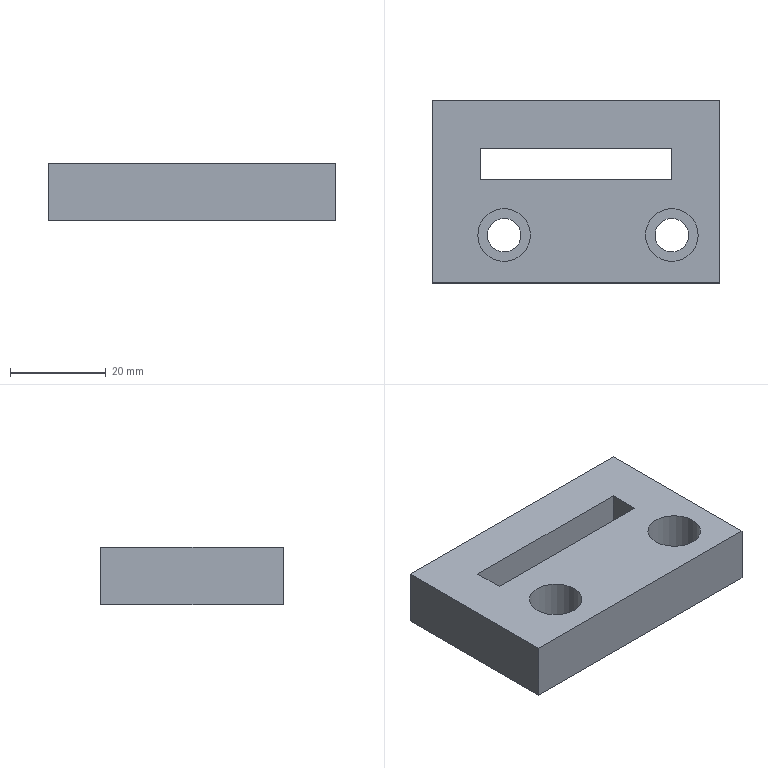Part | STEP file | lll_id682_x_t | 1 solid | 16 faces | box 60 x 38 x 12 mm | volume 22481 mm3 | plane 12 | cylinder 4 | commonest cylinder face diameters 7.009 x2 11.008 x2
STEP:
#1=CARTESIAN_POINT('',(359.5,-168.675,-12.));
#2=VERTEX_POINT('',#1);
#3=CARTESIAN_POINT('',(359.5,-162.325,-12.));
#4=VERTEX_POINT('',#3);
#5=CARTESIAN_POINT('',(359.5,-168.675,-12.));
#6=DIRECTION('',(0.,1.,0.));
#7=VECTOR('',#6,1.);
#8=LINE('',#5,#7);
#9=EDGE_CURVE('',#2,#4,#8,.T.);
#10=ORIENTED_EDGE('',*,*,#9,.T.);
#11=CARTESIAN_POINT('',(319.5,-162.325,-12.));
#12=VERTEX_POINT('',#11);
#13=CARTESIAN_POINT('',(339.5,-162.325,-12.));
#14=DIRECTION('',(-1.,0.,0.));
#15=VECTOR('',#14,1.);
#16=LINE('',#13,#15);
#17=EDGE_CURVE('',#4,#12,#16,.T.);
#18=ORIENTED_EDGE('',*,*,#17,.T.);
#19=CARTESIAN_POINT('',(319.5,-168.675,-12.));
#20=VERTEX_POINT('',#19);
#21=CARTESIAN_POINT('',(319.5,-168.675,-12.));
#22=DIRECTION('',(0.,1.,0.));
#23=VECTOR('',#22,1.);
#24=LINE('',#21,#23);
#25=EDGE_CURVE('',#20,#12,#24,.T.);
#26=ORIENTED_EDGE('',*,*,#25,.F.);
#27=CARTESIAN_POINT('',(339.5,-168.675,-12.));
#28=DIRECTION('',(-1.,0.,0.));
#29=VECTOR('',#28,1.);
#30=LINE('',#27,#29);
#31=EDGE_CURVE('',#2,#20,#30,.T.);
#32=ORIENTED_EDGE('',*,*,#31,.F.);
#33=EDGE_LOOP('',(#10,#18,#26,#32));
#34=FACE_BOUND('',#33,.T.);
#35=CARTESIAN_POINT('',(369.505,-190.325,-12.));
#36=VERTEX_POINT('',#35);
#37=CARTESIAN_POINT('',(369.505,-152.325,-12.));
#38=VERTEX_POINT('',#37);
#39=CARTESIAN_POINT('',(369.505,-165.5,-12.));
#40=DIRECTION('',(0.,1.,0.));
#41=VECTOR('',#40,1.);
#42=LINE('',#39,#41);
#43=EDGE_CURVE('',#36,#38,#42,.T.);
#44=ORIENTED_EDGE('',*,*,#43,.F.);
#45=CARTESIAN_POINT('',(309.505,-190.325,-12.));
#46=VERTEX_POINT('',#45);
#47=CARTESIAN_POINT('',(44.,-190.325,-12.));
#48=DIRECTION('',(1.,0.,0.));
#49=VECTOR('',#48,1.);
#50=LINE('',#47,#49);
#51=EDGE_CURVE('',#46,#36,#50,.T.);
#52=ORIENTED_EDGE('',*,*,#51,.F.);
#53=CARTESIAN_POINT('',(309.505,-152.325,-12.));
#54=VERTEX_POINT('',#53);
#55=CARTESIAN_POINT('',(309.505,-165.5,-12.));
#56=DIRECTION('',(0.,-1.,0.));
#57=VECTOR('',#56,1.);
#58=LINE('',#55,#57);
#59=EDGE_CURVE('',#54,#46,#58,.T.);
#60=ORIENTED_EDGE('',*,*,#59,.F.);
#61=CARTESIAN_POINT('',(44.,-152.325,-12.));
#62=DIRECTION('',(-1.,0.,0.));
#63=VECTOR('',#62,1.);
#64=LINE('',#61,#63);
#65=EDGE_CURVE('',#38,#54,#64,.T.);
#66=ORIENTED_EDGE('',*,*,#65,.F.);
#67=EDGE_LOOP('',(#44,#52,#60,#66));
#68=FACE_BOUND('',#67,.T.);
#69=CARTESIAN_POINT('',(328.009,-180.325,-12.));
#70=VERTEX_POINT('',#69);
#71=CARTESIAN_POINT('',(324.505,-180.325,-12.));
#72=DIRECTION('',(0.,0.,-1.));
#73=DIRECTION('',(1.,0.,0.));
#74=AXIS2_PLACEMENT_3D('',#71,#72,#73);
#75=CIRCLE('',#74,3.505);
#76=EDGE_CURVE('',#70,#70,#75,.T.);
#77=ORIENTED_EDGE('',*,*,#76,.F.);
#78=EDGE_LOOP('',(#77));
#79=FACE_BOUND('',#78,.T.);
#80=CARTESIAN_POINT('',(356.,-180.325,-12.));
#81=VERTEX_POINT('',#80);
#82=CARTESIAN_POINT('',(359.505,-180.325,-12.));
#83=DIRECTION('',(0.,0.,1.));
#84=DIRECTION('',(-1.,0.,0.));
#85=AXIS2_PLACEMENT_3D('',#82,#83,#84);
#86=CIRCLE('',#85,3.505);
#87=EDGE_CURVE('',#81,#81,#86,.T.);
#88=ORIENTED_EDGE('',*,*,#87,.T.);
#89=EDGE_LOOP('',(#88));
#90=FACE_BOUND('',#89,.T.);
#91=CARTESIAN_POINT('',(329.505,-165.5,-12.));
#92=DIRECTION('',(0.,0.,-1.));
#93=DIRECTION('',(1.,0.,0.));
#94=AXIS2_PLACEMENT_3D('',#91,#92,#93);
#95=PLANE('',#94);
#96=ADVANCED_FACE('',(#34,#68,#79,#90),#95,.T.);
#97=CARTESIAN_POINT('',(369.505,-190.325,0.));
#98=VERTEX_POINT('',#97);
#99=CARTESIAN_POINT('',(309.505,-190.325,0.));
#100=VERTEX_POINT('',#99);
#101=CARTESIAN_POINT('',(44.,-190.325,0.));
#102=DIRECTION('',(-1.,0.,0.));
#103=VECTOR('',#102,1.);
#104=LINE('',#101,#103);
#105=EDGE_CURVE('',#98,#100,#104,.T.);
#106=ORIENTED_EDGE('',*,*,#105,.F.);
#107=CARTESIAN_POINT('',(369.505,-152.325,0.));
#108=VERTEX_POINT('',#107);
#109=CARTESIAN_POINT('',(369.505,-165.5,0.));
#110=DIRECTION('',(0.,-1.,0.));
#111=VECTOR('',#110,1.);
#112=LINE('',#109,#111);
#113=EDGE_CURVE('',#108,#98,#112,.T.);
#114=ORIENTED_EDGE('',*,*,#113,.F.);
#115=CARTESIAN_POINT('',(309.505,-152.325,0.));
#116=VERTEX_POINT('',#115);
#117=CARTESIAN_POINT('',(44.,-152.325,0.));
#118=DIRECTION('',(1.,0.,0.));
#119=VECTOR('',#118,1.);
#120=LINE('',#117,#119);
#121=EDGE_CURVE('',#116,#108,#120,.T.);
#122=ORIENTED_EDGE('',*,*,#121,.F.);
#123=CARTESIAN_POINT('',(309.505,-165.5,0.));
#124=DIRECTION('',(0.,1.,0.));
#125=VECTOR('',#124,1.);
#126=LINE('',#123,#125);
#127=EDGE_CURVE('',#100,#116,#126,.T.);
#128=ORIENTED_EDGE('',*,*,#127,.F.);
#129=EDGE_LOOP('',(#106,#114,#122,#128));
#130=FACE_BOUND('',#129,.T.);
#131=CARTESIAN_POINT('',(359.5,-162.325,0.));
#132=VERTEX_POINT('',#131);
#133=CARTESIAN_POINT('',(319.5,-162.325,0.));
#134=VERTEX_POINT('',#133);
#135=CARTESIAN_POINT('',(339.5,-162.325,0.));
#136=DIRECTION('',(-1.,0.,0.));
#137=VECTOR('',#136,1.);
#138=LINE('',#135,#137);
#139=EDGE_CURVE('',#132,#134,#138,.T.);
#140=ORIENTED_EDGE('',*,*,#139,.F.);
#141=CARTESIAN_POINT('',(359.5,-168.675,0.));
#142=VERTEX_POINT('',#141);
#143=CARTESIAN_POINT('',(359.5,-168.675,0.));
#144=DIRECTION('',(0.,1.,0.));
#145=VECTOR('',#144,1.);
#146=LINE('',#143,#145);
#147=EDGE_CURVE('',#142,#132,#146,.T.);
#148=ORIENTED_EDGE('',*,*,#147,.F.);
#149=CARTESIAN_POINT('',(319.5,-168.675,0.));
#150=VERTEX_POINT('',#149);
#151=CARTESIAN_POINT('',(339.5,-168.675,0.));
#152=DIRECTION('',(-1.,0.,0.));
#153=VECTOR('',#152,1.);
#154=LINE('',#151,#153);
#155=EDGE_CURVE('',#142,#150,#154,.T.);
#156=ORIENTED_EDGE('',*,*,#155,.T.);
#157=CARTESIAN_POINT('',(319.5,-168.675,0.));
#158=DIRECTION('',(0.,1.,0.));
#159=VECTOR('',#158,1.);
#160=LINE('',#157,#159);
#161=EDGE_CURVE('',#150,#134,#160,.T.);
#162=ORIENTED_EDGE('',*,*,#161,.T.);
#163=EDGE_LOOP('',(#140,#148,#156,#162));
#164=FACE_BOUND('',#163,.T.);
#165=CARTESIAN_POINT('',(330.009,-180.325,0.));
#166=VERTEX_POINT('',#165);
#167=CARTESIAN_POINT('',(324.505,-180.325,0.));
#168=DIRECTION('',(0.,0.,1.));
#169=DIRECTION('',(1.,0.,0.));
#170=AXIS2_PLACEMENT_3D('',#167,#168,#169);
#171=CIRCLE('',#170,5.504);
#172=EDGE_CURVE('',#166,#166,#171,.T.);
#173=ORIENTED_EDGE('',*,*,#172,.F.);
#174=EDGE_LOOP('',(#173));
#175=FACE_BOUND('',#174,.T.);
#176=CARTESIAN_POINT('',(354.001,-180.325,0.));
#177=VERTEX_POINT('',#176);
#178=CARTESIAN_POINT('',(359.505,-180.325,0.));
#179=DIRECTION('',(0.,0.,-1.));
#180=DIRECTION('',(-1.,0.,0.));
#181=AXIS2_PLACEMENT_3D('',#178,#179,#180);
#182=CIRCLE('',#181,5.504);
#183=EDGE_CURVE('',#177,#177,#182,.T.);
#184=ORIENTED_EDGE('',*,*,#183,.T.);
#185=EDGE_LOOP('',(#184));
#186=FACE_BOUND('',#185,.T.);
#187=CARTESIAN_POINT('',(329.505,-165.5,0.));
#188=DIRECTION('',(0.,0.,1.));
#189=DIRECTION('',(-1.,0.,0.));
#190=AXIS2_PLACEMENT_3D('',#187,#188,#189);
#191=PLANE('',#190);
#192=ADVANCED_FACE('',(#130,#164,#175,#186),#191,.T.);
#193=CARTESIAN_POINT('',(369.505,-190.325,0.));
#194=DIRECTION('',(0.,0.,1.));
#195=VECTOR('',#194,1.);
#196=LINE('',#193,#195);
#197=EDGE_CURVE('',#36,#98,#196,.T.);
#198=ORIENTED_EDGE('',*,*,#197,.T.);
#199=ORIENTED_EDGE('',*,*,#105,.T.);
#200=CARTESIAN_POINT('',(309.505,-190.325,-12.));
#201=DIRECTION('',(0.,0.,1.));
#202=VECTOR('',#201,1.);
#203=LINE('',#200,#202);
#204=EDGE_CURVE('',#46,#100,#203,.T.);
#205=ORIENTED_EDGE('',*,*,#204,.F.);
#206=ORIENTED_EDGE('',*,*,#51,.T.);
#207=EDGE_LOOP('',(#198,#199,#205,#206));
#208=FACE_OUTER_BOUND('',#207,.T.);
#209=CARTESIAN_POINT('',(44.,-190.325,0.));
#210=DIRECTION('',(0.,-1.,0.));
#211=DIRECTION('',(0.,0.,1.));
#212=AXIS2_PLACEMENT_3D('',#209,#210,#211);
#213=PLANE('',#212);
#214=ADVANCED_FACE('',(#208),#213,.T.);
#215=ORIENTED_EDGE('',*,*,#204,.T.);
#216=ORIENTED_EDGE('',*,*,#127,.T.);
#217=CARTESIAN_POINT('',(309.505,-152.325,0.));
#218=DIRECTION('',(0.,0.,1.));
#219=VECTOR('',#218,1.);
#220=LINE('',#217,#219);
#221=EDGE_CURVE('',#54,#116,#220,.T.);
#222=ORIENTED_EDGE('',*,*,#221,.F.);
#223=ORIENTED_EDGE('',*,*,#59,.T.);
#224=EDGE_LOOP('',(#215,#216,#222,#223));
#225=FACE_OUTER_BOUND('',#224,.T.);
#226=CARTESIAN_POINT('',(309.505,-165.5,-12.));
#227=DIRECTION('',(-1.,0.,0.));
#228=DIRECTION('',(0.,0.,-1.));
#229=AXIS2_PLACEMENT_3D('',#226,#227,#228);
#230=PLANE('',#229);
#231=ADVANCED_FACE('',(#225),#230,.T.);
#232=ORIENTED_EDGE('',*,*,#221,.T.);
#233=ORIENTED_EDGE('',*,*,#121,.T.);
#234=CARTESIAN_POINT('',(369.505,-152.325,-12.));
#235=DIRECTION('',(0.,0.,1.));
#236=VECTOR('',#235,1.);
#237=LINE('',#234,#236);
#238=EDGE_CURVE('',#38,#108,#237,.T.);
#239=ORIENTED_EDGE('',*,*,#238,.F.);
#240=ORIENTED_EDGE('',*,*,#65,.T.);
#241=EDGE_LOOP('',(#232,#233,#239,#240));
#242=FACE_OUTER_BOUND('',#241,.T.);
#243=CARTESIAN_POINT('',(44.,-152.325,0.));
#244=DIRECTION('',(0.,-1.,0.));
#245=DIRECTION('',(0.,0.,1.));
#246=AXIS2_PLACEMENT_3D('',#243,#244,#245);
#247=PLANE('',#246);
#248=ADVANCED_FACE('',(#242),#247,.F.);
#249=ORIENTED_EDGE('',*,*,#43,.T.);
#250=ORIENTED_EDGE('',*,*,#238,.T.);
#251=ORIENTED_EDGE('',*,*,#113,.T.);
#252=ORIENTED_EDGE('',*,*,#197,.F.);
#253=EDGE_LOOP('',(#249,#250,#251,#252));
#254=FACE_OUTER_BOUND('',#253,.T.);
#255=CARTESIAN_POINT('',(369.505,-165.5,-12.));
#256=DIRECTION('',(1.,0.,0.));
#257=DIRECTION('',(0.,0.,1.));
#258=AXIS2_PLACEMENT_3D('',#255,#256,#257);
#259=PLANE('',#258);
#260=ADVANCED_FACE('',(#254),#259,.T.);
#261=CARTESIAN_POINT('',(319.5,-162.325,-12.));
#262=DIRECTION('',(0.,0.,-1.));
#263=VECTOR('',#262,1.);
#264=LINE('',#261,#263);
#265=EDGE_CURVE('',#134,#12,#264,.T.);
#266=ORIENTED_EDGE('',*,*,#265,.F.);
#267=ORIENTED_EDGE('',*,*,#161,.F.);
#268=CARTESIAN_POINT('',(319.5,-168.675,-12.));
#269=DIRECTION('',(0.,0.,-1.));
#270=VECTOR('',#269,1.);
#271=LINE('',#268,#270);
#272=EDGE_CURVE('',#150,#20,#271,.T.);
#273=ORIENTED_EDGE('',*,*,#272,.T.);
#274=ORIENTED_EDGE('',*,*,#25,.T.);
#275=EDGE_LOOP('',(#266,#267,#273,#274));
#276=FACE_OUTER_BOUND('',#275,.T.);
#277=CARTESIAN_POINT('',(319.5,-168.675,-12.));
#278=DIRECTION('',(-1.,0.,0.));
#279=DIRECTION('',(0.,0.,-1.));
#280=AXIS2_PLACEMENT_3D('',#277,#278,#279);
#281=PLANE('',#280);
#282=ADVANCED_FACE('',(#276),#281,.F.);
#283=CARTESIAN_POINT('',(359.5,-162.325,-12.));
#284=DIRECTION('',(0.,0.,-1.));
#285=VECTOR('',#284,1.);
#286=LINE('',#283,#285);
#287=EDGE_CURVE('',#132,#4,#286,.T.);
#288=ORIENTED_EDGE('',*,*,#287,.T.);
#289=ORIENTED_EDGE('',*,*,#9,.F.);
#290=CARTESIAN_POINT('',(359.5,-168.675,-12.));
#291=DIRECTION('',(0.,0.,-1.));
#292=VECTOR('',#291,1.);
#293=LINE('',#290,#292);
#294=EDGE_CURVE('',#142,#2,#293,.T.);
#295=ORIENTED_EDGE('',*,*,#294,.F.);
#296=ORIENTED_EDGE('',*,*,#147,.T.);
#297=EDGE_LOOP('',(#288,#289,#295,#296));
#298=FACE_OUTER_BOUND('',#297,.T.);
#299=CARTESIAN_POINT('',(359.5,-168.675,-12.));
#300=DIRECTION('',(-1.,0.,0.));
#301=DIRECTION('',(0.,0.,-1.));
#302=AXIS2_PLACEMENT_3D('',#299,#300,#301);
#303=PLANE('',#302);
#304=ADVANCED_FACE('',(#298),#303,.T.);
#305=ORIENTED_EDGE('',*,*,#272,.F.);
#306=ORIENTED_EDGE('',*,*,#155,.F.);
#307=ORIENTED_EDGE('',*,*,#294,.T.);
#308=ORIENTED_EDGE('',*,*,#31,.T.);
#309=EDGE_LOOP('',(#305,#306,#307,#308));
#310=FACE_OUTER_BOUND('',#309,.T.);
#311=CARTESIAN_POINT('',(44.,-168.675,0.));
#312=DIRECTION('',(0.,-1.,0.));
#313=DIRECTION('',(0.,0.,1.));
#314=AXIS2_PLACEMENT_3D('',#311,#312,#313);
#315=PLANE('',#314);
#316=ADVANCED_FACE('',(#310),#315,.F.);
#317=ORIENTED_EDGE('',*,*,#265,.T.);
#318=ORIENTED_EDGE('',*,*,#17,.F.);
#319=ORIENTED_EDGE('',*,*,#287,.F.);
#320=ORIENTED_EDGE('',*,*,#139,.T.);
#321=EDGE_LOOP('',(#317,#318,#319,#320));
#322=FACE_OUTER_BOUND('',#321,.T.);
#323=CARTESIAN_POINT('',(44.,-162.325,0.));
#324=DIRECTION('',(0.,-1.,0.));
#325=DIRECTION('',(0.,0.,1.));
#326=AXIS2_PLACEMENT_3D('',#323,#324,#325);
#327=PLANE('',#326);
#328=ADVANCED_FACE('',(#322),#327,.T.);
#329=CARTESIAN_POINT('',(328.009,-180.325,-8.));
#330=VERTEX_POINT('',#329);
#331=CARTESIAN_POINT('',(324.505,-180.325,-8.));
#332=DIRECTION('',(0.,0.,1.));
#333=DIRECTION('',(1.,0.,0.));
#334=AXIS2_PLACEMENT_3D('',#331,#332,#333);
#335=CIRCLE('',#334,3.505);
#336=EDGE_CURVE('',#330,#330,#335,.T.);
#337=ORIENTED_EDGE('',*,*,#336,.T.);
#338=EDGE_LOOP('',(#337));
#339=FACE_BOUND('',#338,.T.);
#340=ORIENTED_EDGE('',*,*,#76,.T.);
#341=EDGE_LOOP('',(#340));
#342=FACE_BOUND('',#341,.T.);
#343=CARTESIAN_POINT('',(324.505,-180.325,0.));
#344=DIRECTION('',(0.,0.,-1.));
#345=DIRECTION('',(-1.,0.,0.));
#346=AXIS2_PLACEMENT_3D('',#343,#344,#345);
#347=CYLINDRICAL_SURFACE('',#346,3.505);
#348=ADVANCED_FACE('',(#339,#342),#347,.F.);
#349=ORIENTED_EDGE('',*,*,#336,.F.);
#350=EDGE_LOOP('',(#349));
#351=FACE_BOUND('',#350,.T.);
#352=CARTESIAN_POINT('',(330.009,-180.325,-8.));
#353=VERTEX_POINT('',#352);
#354=CARTESIAN_POINT('',(324.505,-180.325,-8.));
#355=DIRECTION('',(0.,0.,1.));
#356=DIRECTION('',(1.,0.,0.));
#357=AXIS2_PLACEMENT_3D('',#354,#355,#356);
#358=CIRCLE('',#357,5.504);
#359=EDGE_CURVE('',#353,#353,#358,.T.);
#360=ORIENTED_EDGE('',*,*,#359,.T.);
#361=EDGE_LOOP('',(#360));
#362=FACE_BOUND('',#361,.T.);
#363=CARTESIAN_POINT('',(324.505,-180.325,-8.));
#364=DIRECTION('',(0.,0.,-1.));
#365=DIRECTION('',(-1.,0.,0.));
#366=AXIS2_PLACEMENT_3D('',#363,#364,#365);
#367=PLANE('',#366);
#368=ADVANCED_FACE('',(#351,#362),#367,.F.);
#369=ORIENTED_EDGE('',*,*,#359,.F.);
#370=EDGE_LOOP('',(#369));
#371=FACE_BOUND('',#370,.T.);
#372=ORIENTED_EDGE('',*,*,#172,.T.);
#373=EDGE_LOOP('',(#372));
#374=FACE_BOUND('',#373,.T.);
#375=CARTESIAN_POINT('',(324.505,-180.325,0.));
#376=DIRECTION('',(0.,0.,-1.));
#377=DIRECTION('',(-1.,0.,0.));
#378=AXIS2_PLACEMENT_3D('',#375,#376,#377);
#379=CYLINDRICAL_SURFACE('',#378,5.504);
#380=ADVANCED_FACE('',(#371,#374),#379,.F.);
#381=CARTESIAN_POINT('',(356.,-180.325,-8.));
#382=VERTEX_POINT('',#381);
#383=CARTESIAN_POINT('',(359.505,-180.325,-8.));
#384=DIRECTION('',(0.,0.,-1.));
#385=DIRECTION('',(-1.,0.,0.));
#386=AXIS2_PLACEMENT_3D('',#383,#384,#385);
#387=CIRCLE('',#386,3.505);
#388=EDGE_CURVE('',#382,#382,#387,.T.);
#389=ORIENTED_EDGE('',*,*,#388,.F.);
#390=EDGE_LOOP('',(#389));
#391=FACE_BOUND('',#390,.T.);
#392=ORIENTED_EDGE('',*,*,#87,.F.);
#393=EDGE_LOOP('',(#392));
#394=FACE_BOUND('',#393,.T.);
#395=CARTESIAN_POINT('',(359.505,-180.325,0.));
#396=DIRECTION('',(0.,0.,-1.));
#397=DIRECTION('',(1.,0.,0.));
#398=AXIS2_PLACEMENT_3D('',#395,#396,#397);
#399=CYLINDRICAL_SURFACE('',#398,3.505);
#400=ADVANCED_FACE('',(#391,#394),#399,.F.);
#401=ORIENTED_EDGE('',*,*,#388,.T.);
#402=EDGE_LOOP('',(#401));
#403=FACE_BOUND('',#402,.T.);
#404=CARTESIAN_POINT('',(354.001,-180.325,-8.));
#405=VERTEX_POINT('',#404);
#406=CARTESIAN_POINT('',(359.505,-180.325,-8.));
#407=DIRECTION('',(0.,0.,-1.));
#408=DIRECTION('',(-1.,0.,0.));
#409=AXIS2_PLACEMENT_3D('',#406,#407,#408);
#410=CIRCLE('',#409,5.504);
#411=EDGE_CURVE('',#405,#405,#410,.T.);
#412=ORIENTED_EDGE('',*,*,#411,.F.);
#413=EDGE_LOOP('',(#412));
#414=FACE_BOUND('',#413,.T.);
#415=CARTESIAN_POINT('',(359.505,-180.325,-8.));
#416=DIRECTION('',(0.,0.,-1.));
#417=DIRECTION('',(1.,0.,0.));
#418=AXIS2_PLACEMENT_3D('',#415,#416,#417);
#419=PLANE('',#418);
#420=ADVANCED_FACE('',(#403,#414),#419,.F.);
#421=ORIENTED_EDGE('',*,*,#411,.T.);
#422=EDGE_LOOP('',(#421));
#423=FACE_BOUND('',#422,.T.);
#424=ORIENTED_EDGE('',*,*,#183,.F.);
#425=EDGE_LOOP('',(#424));
#426=FACE_BOUND('',#425,.T.);
#427=CARTESIAN_POINT('',(359.505,-180.325,0.));
#428=DIRECTION('',(0.,0.,-1.));
#429=DIRECTION('',(1.,0.,0.));
#430=AXIS2_PLACEMENT_3D('',#427,#428,#429);
#431=CYLINDRICAL_SURFACE('',#430,5.504);
#432=ADVANCED_FACE('',(#423,#426),#431,.F.);
#433=CLOSED_SHELL('',(#96,#192,#214,#231,#248,#260,#282,#304,#316,#328,#348,#368,#380,#400,#420,#432));
#434=MANIFOLD_SOLID_BREP('',#433);
#435=(LENGTH_UNIT()NAMED_UNIT(*)SI_UNIT(.MILLI.,.METRE.));
#436=UNCERTAINTY_MEASURE_WITH_UNIT(LENGTH_MEASURE(0.00002),#435,'','');
#437=(NAMED_UNIT(*)PLANE_ANGLE_UNIT()SI_UNIT($,.RADIAN.));
#438=PLANE_ANGLE_MEASURE_WITH_UNIT(PLANE_ANGLE_MEASURE(0.01745),#437);
#439=DIMENSIONAL_EXPONENTS(0.,0.,0.,0.,0.,0.,0.);
#440=(CONVERSION_BASED_UNIT('DEGREE',#438)NAMED_UNIT(#439)PLANE_ANGLE_UNIT());
#441=(NAMED_UNIT(*)SI_UNIT($,.STERADIAN.)SOLID_ANGLE_UNIT());
#442=(GEOMETRIC_REPRESENTATION_CONTEXT(3)GLOBAL_UNCERTAINTY_ASSIGNED_CONTEXT((#436))GLOBAL_UNIT_ASSIGNED_CONTEXT((#435,#440,#441))REPRESENTATION_CONTEXT('',''));
#443=ADVANCED_BREP_SHAPE_REPRESENTATION('',(#434),#442);